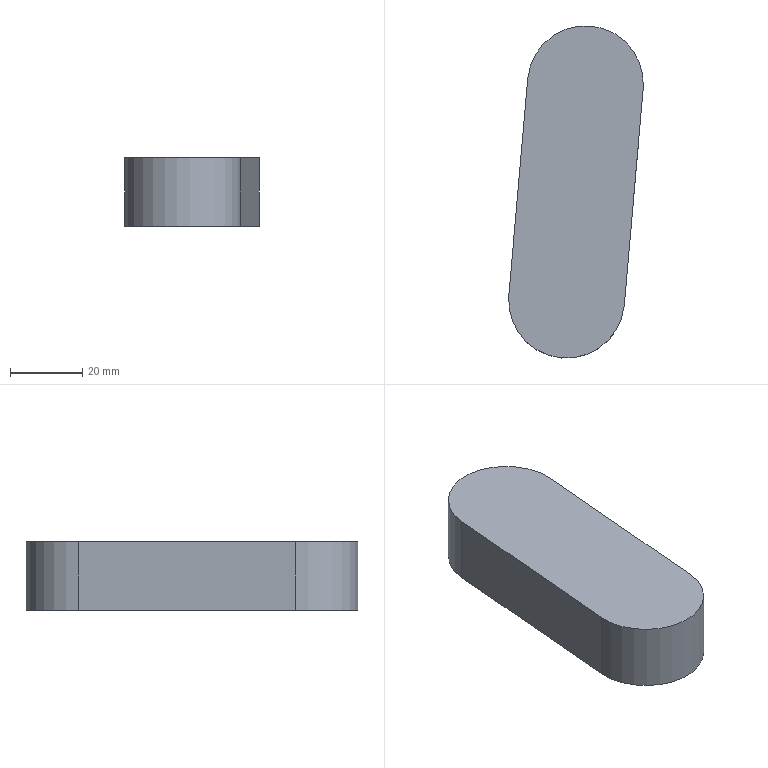Part | NX | features solid 2 | 1 solid | 6 faces | box 37.229 x 91.772 x 19 mm | volume 51761 mm3 | plane 4 | cylinder 2 | commonest cylinder face diameters 32 x2
STEP:
#1=CARTESIAN_POINT('',(523.873,44.511,271.));
#2=VERTEX_POINT('',#1);
#3=CARTESIAN_POINT('',(529.102,104.283,271.));
#4=VERTEX_POINT('',#3);
#5=CARTESIAN_POINT('',(523.873,44.511,271.));
#6=DIRECTION('',(0.08716,0.9962,0.));
#7=VECTOR('',#6,1000.);
#8=LINE('',#5,#7);
#9=EDGE_CURVE('',#2,#4,#8,.T.);
#10=ORIENTED_EDGE('',*,*,#9,.F.);
#11=CARTESIAN_POINT('',(523.873,44.511,252.));
#12=VERTEX_POINT('',#11);
#13=CARTESIAN_POINT('',(523.873,44.511,252.));
#14=DIRECTION('',(0.,0.,1.));
#15=VECTOR('',#14,1000.);
#16=LINE('',#13,#15);
#17=EDGE_CURVE('',#2,#12,#16,.F.);
#18=ORIENTED_EDGE('',*,*,#17,.T.);
#19=CARTESIAN_POINT('',(529.102,104.283,252.));
#20=VERTEX_POINT('',#19);
#21=CARTESIAN_POINT('',(523.873,44.511,252.));
#22=DIRECTION('',(0.08716,0.9962,0.));
#23=VECTOR('',#22,1000.);
#24=LINE('',#21,#23);
#25=EDGE_CURVE('',#12,#20,#24,.T.);
#26=ORIENTED_EDGE('',*,*,#25,.T.);
#27=CARTESIAN_POINT('',(529.102,104.283,252.));
#28=DIRECTION('',(0.,0.,1.));
#29=VECTOR('',#28,1000.);
#30=LINE('',#27,#29);
#31=EDGE_CURVE('',#20,#4,#30,.T.);
#32=ORIENTED_EDGE('',*,*,#31,.T.);
#33=EDGE_LOOP('',(#10,#18,#26,#32));
#34=FACE_BOUND('',#33,.T.);
#35=CARTESIAN_POINT('',(523.873,44.511,252.));
#36=DIRECTION('',(0.9962,-0.08716,0.));
#37=DIRECTION('',(0.08716,0.9962,0.));
#38=AXIS2_PLACEMENT_3D('',#35,#36,#37);
#39=PLANE('',#38);
#40=ADVANCED_FACE('',(#34),#39,.T.);
#41=CARTESIAN_POINT('',(491.995,47.3,252.));
#42=VERTEX_POINT('',#41);
#43=CARTESIAN_POINT('',(497.224,107.072,252.));
#44=VERTEX_POINT('',#43);
#45=CARTESIAN_POINT('',(491.995,47.3,252.));
#46=DIRECTION('',(0.08716,0.9962,0.));
#47=VECTOR('',#46,1000.);
#48=LINE('',#45,#47);
#49=EDGE_CURVE('',#42,#44,#48,.T.);
#50=ORIENTED_EDGE('',*,*,#49,.F.);
#51=CARTESIAN_POINT('',(491.995,47.3,271.));
#52=VERTEX_POINT('',#51);
#53=CARTESIAN_POINT('',(491.995,47.3,252.));
#54=DIRECTION('',(0.,0.,1.));
#55=VECTOR('',#54,1000.);
#56=LINE('',#53,#55);
#57=EDGE_CURVE('',#42,#52,#56,.T.);
#58=ORIENTED_EDGE('',*,*,#57,.T.);
#59=CARTESIAN_POINT('',(497.224,107.072,271.));
#60=VERTEX_POINT('',#59);
#61=CARTESIAN_POINT('',(491.995,47.3,271.));
#62=DIRECTION('',(0.08716,0.9962,0.));
#63=VECTOR('',#62,1000.);
#64=LINE('',#61,#63);
#65=EDGE_CURVE('',#52,#60,#64,.T.);
#66=ORIENTED_EDGE('',*,*,#65,.T.);
#67=CARTESIAN_POINT('',(497.224,107.072,252.));
#68=DIRECTION('',(0.,0.,1.));
#69=VECTOR('',#68,1000.);
#70=LINE('',#67,#69);
#71=EDGE_CURVE('',#60,#44,#70,.F.);
#72=ORIENTED_EDGE('',*,*,#71,.T.);
#73=EDGE_LOOP('',(#50,#58,#66,#72));
#74=FACE_BOUND('',#73,.T.);
#75=CARTESIAN_POINT('',(491.995,47.3,252.));
#76=DIRECTION('',(0.9962,-0.08716,0.));
#77=DIRECTION('',(0.08716,0.9962,0.));
#78=AXIS2_PLACEMENT_3D('',#75,#76,#77);
#79=PLANE('',#78);
#80=ADVANCED_FACE('',(#74),#79,.F.);
#81=CARTESIAN_POINT('',(507.934,45.905,252.));
#82=DIRECTION('',(0.,0.,-1.));
#83=DIRECTION('',(-0.08716,-0.9962,0.));
#84=AXIS2_PLACEMENT_3D('',#81,#82,#83);
#85=CIRCLE('',#84,16.);
#86=EDGE_CURVE('',#12,#42,#85,.T.);
#87=ORIENTED_EDGE('',*,*,#86,.T.);
#88=ORIENTED_EDGE('',*,*,#49,.T.);
#89=CARTESIAN_POINT('',(513.163,105.677,252.));
#90=DIRECTION('',(0.,0.,-1.));
#91=DIRECTION('',(-0.08716,-0.9962,0.));
#92=AXIS2_PLACEMENT_3D('',#89,#90,#91);
#93=CIRCLE('',#92,16.);
#94=EDGE_CURVE('',#44,#20,#93,.T.);
#95=ORIENTED_EDGE('',*,*,#94,.T.);
#96=ORIENTED_EDGE('',*,*,#25,.F.);
#97=EDGE_LOOP('',(#87,#88,#95,#96));
#98=FACE_BOUND('',#97,.T.);
#99=CARTESIAN_POINT('',(454.139,50.612,252.));
#100=DIRECTION('',(0.,0.,-1.));
#101=DIRECTION('',(-0.08716,-0.9962,0.));
#102=AXIS2_PLACEMENT_3D('',#99,#100,#101);
#103=PLANE('',#102);
#104=ADVANCED_FACE('',(#98),#103,.T.);
#105=ORIENTED_EDGE('',*,*,#65,.F.);
#106=CARTESIAN_POINT('',(507.934,45.905,271.));
#107=DIRECTION('',(0.,0.,-1.));
#108=DIRECTION('',(-0.08716,-0.9962,0.));
#109=AXIS2_PLACEMENT_3D('',#106,#107,#108);
#110=CIRCLE('',#109,16.);
#111=EDGE_CURVE('',#52,#2,#110,.F.);
#112=ORIENTED_EDGE('',*,*,#111,.T.);
#113=ORIENTED_EDGE('',*,*,#9,.T.);
#114=CARTESIAN_POINT('',(513.163,105.677,271.));
#115=DIRECTION('',(0.,0.,-1.));
#116=DIRECTION('',(-0.08716,-0.9962,0.));
#117=AXIS2_PLACEMENT_3D('',#114,#115,#116);
#118=CIRCLE('',#117,16.);
#119=EDGE_CURVE('',#4,#60,#118,.F.);
#120=ORIENTED_EDGE('',*,*,#119,.T.);
#121=EDGE_LOOP('',(#105,#112,#113,#120));
#122=FACE_BOUND('',#121,.T.);
#123=CARTESIAN_POINT('',(454.139,50.612,271.));
#124=DIRECTION('',(0.,0.,-1.));
#125=DIRECTION('',(-0.08716,-0.9962,0.));
#126=AXIS2_PLACEMENT_3D('',#123,#124,#125);
#127=PLANE('',#126);
#128=ADVANCED_FACE('',(#122),#127,.F.);
#129=ORIENTED_EDGE('',*,*,#111,.F.);
#130=ORIENTED_EDGE('',*,*,#57,.F.);
#131=ORIENTED_EDGE('',*,*,#86,.F.);
#132=ORIENTED_EDGE('',*,*,#17,.F.);
#133=EDGE_LOOP('',(#129,#130,#131,#132));
#134=FACE_BOUND('',#133,.T.);
#135=CARTESIAN_POINT('',(507.934,45.905,252.));
#136=DIRECTION('',(0.,0.,-1.));
#137=DIRECTION('',(-0.08716,-0.9962,0.));
#138=AXIS2_PLACEMENT_3D('',#135,#136,#137);
#139=CYLINDRICAL_SURFACE('',#138,16.);
#140=ADVANCED_FACE('',(#134),#139,.T.);
#141=ORIENTED_EDGE('',*,*,#31,.F.);
#142=ORIENTED_EDGE('',*,*,#94,.F.);
#143=ORIENTED_EDGE('',*,*,#71,.F.);
#144=ORIENTED_EDGE('',*,*,#119,.F.);
#145=EDGE_LOOP('',(#141,#142,#143,#144));
#146=FACE_BOUND('',#145,.T.);
#147=CARTESIAN_POINT('',(513.163,105.677,252.));
#148=DIRECTION('',(0.,0.,1.));
#149=DIRECTION('',(0.08716,0.9962,0.));
#150=AXIS2_PLACEMENT_3D('',#147,#148,#149);
#151=CYLINDRICAL_SURFACE('',#150,16.);
#152=ADVANCED_FACE('',(#146),#151,.T.);
#153=CLOSED_SHELL('',(#40,#80,#104,#128,#140,#152));
#154=MANIFOLD_SOLID_BREP('',#153);
#155=(LENGTH_UNIT()NAMED_UNIT(*)SI_UNIT(.MILLI.,.METRE.));
#156=UNCERTAINTY_MEASURE_WITH_UNIT(LENGTH_MEASURE(0.00001),#155,'','');
#157=(NAMED_UNIT(*)PLANE_ANGLE_UNIT()SI_UNIT($,.RADIAN.));
#158=(NAMED_UNIT(*)SI_UNIT($,.STERADIAN.)SOLID_ANGLE_UNIT());
#159=(GEOMETRIC_REPRESENTATION_CONTEXT(3)GLOBAL_UNCERTAINTY_ASSIGNED_CONTEXT((#156))GLOBAL_UNIT_ASSIGNED_CONTEXT((#155,#157,#158))REPRESENTATION_CONTEXT('',''));
#160=ADVANCED_BREP_SHAPE_REPRESENTATION('',(#154),#159);